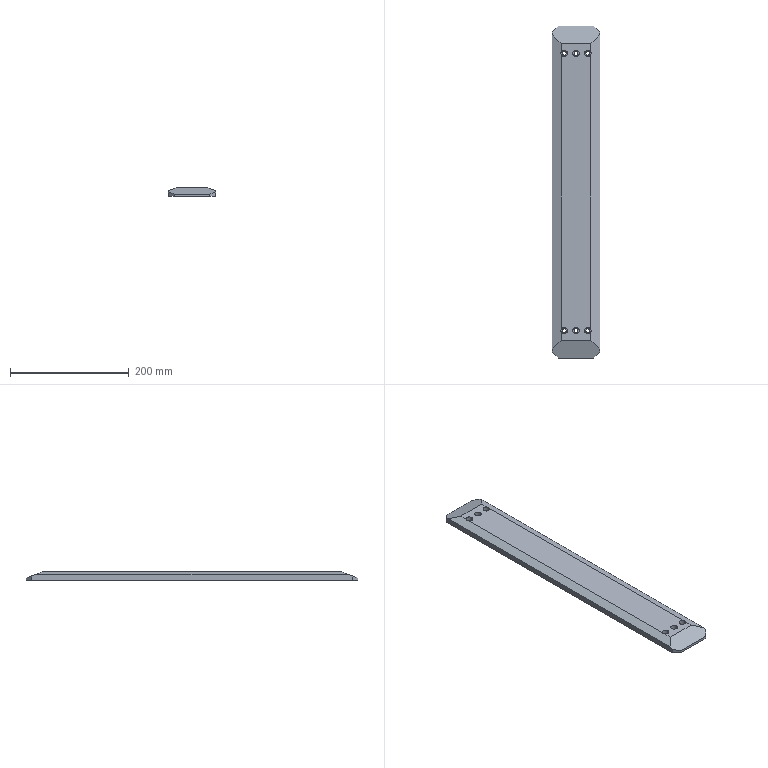Part | SolidWorks | features BaseBody 1 | 1 solid | 44 faces | box 80 x 560 x 15 mm | volume 596607 mm3 | cylinder 24 | plane 20 | commonest cylinder face diameters 6.6 x12 11 x12
STEP:
#1=CARTESIAN_POINT('',(14.5,-234.,6.));
#2=VERTEX_POINT('',#1);
#3=CARTESIAN_POINT('',(25.5,-234.,6.));
#4=VERTEX_POINT('',#3);
#5=CARTESIAN_POINT('',(20.,-234.,6.));
#6=DIRECTION('',(0.,0.,1.));
#7=DIRECTION('',(1.,0.,0.));
#8=AXIS2_PLACEMENT_3D('',#5,#6,#7);
#9=CIRCLE('',#8,5.5);
#10=EDGE_CURVE('',#2,#4,#9,.T.);
#11=ORIENTED_EDGE('',*,*,#10,.F.);
#12=CARTESIAN_POINT('',(14.5,-234.,15.));
#13=VERTEX_POINT('',#12);
#14=CARTESIAN_POINT('',(14.5,-234.,15.));
#15=DIRECTION('',(0.,0.,1.));
#16=VECTOR('',#15,1000.);
#17=LINE('',#14,#16);
#18=EDGE_CURVE('',#2,#13,#17,.T.);
#19=ORIENTED_EDGE('',*,*,#18,.T.);
#20=CARTESIAN_POINT('',(25.,-236.291,15.));
#21=VERTEX_POINT('',#20);
#22=CARTESIAN_POINT('',(20.,-234.,15.));
#23=DIRECTION('',(0.,0.,1.));
#24=DIRECTION('',(1.,0.,0.));
#25=AXIS2_PLACEMENT_3D('',#22,#23,#24);
#26=CIRCLE('',#25,5.5);
#27=EDGE_CURVE('',#13,#21,#26,.T.);
#28=ORIENTED_EDGE('',*,*,#27,.T.);
#29=CARTESIAN_POINT('',(25.5,-234.,14.818));
#30=VERTEX_POINT('',#29);
#31=CARTESIAN_POINT('',(25.,-236.291,15.));
#32=CARTESIAN_POINT('',(25.331,-235.57,14.88));
#33=CARTESIAN_POINT('',(25.5,-234.794,14.818));
#34=CARTESIAN_POINT('',(25.5,-234.,14.818));
#35=(BOUNDED_CURVE()B_SPLINE_CURVE(3,(#31,#32,#33,#34),.UNSPECIFIED.,.F.,.T.)B_SPLINE_CURVE_WITH_KNOTS((4,4),(2.712,3.142),.UNSPECIFIED.)CURVE()GEOMETRIC_REPRESENTATION_ITEM()RATIONAL_B_SPLINE_CURVE((1.,0.9847,0.9847,1.))REPRESENTATION_ITEM(''));
#36=EDGE_CURVE('',#21,#30,#35,.T.);
#37=ORIENTED_EDGE('',*,*,#36,.T.);
#38=CARTESIAN_POINT('',(25.5,-234.,15.));
#39=DIRECTION('',(0.,0.,1.));
#40=VECTOR('',#39,1000.);
#41=LINE('',#38,#40);
#42=EDGE_CURVE('',#4,#30,#41,.T.);
#43=ORIENTED_EDGE('',*,*,#42,.F.);
#44=EDGE_LOOP('',(#11,#19,#28,#37,#43));
#45=FACE_OUTER_BOUND('',#44,.T.);
#46=CARTESIAN_POINT('',(20.,-234.,15.));
#47=DIRECTION('',(0.,0.,1.));
#48=DIRECTION('',(1.,0.,0.));
#49=AXIS2_PLACEMENT_3D('',#46,#47,#48);
#50=CYLINDRICAL_SURFACE('',#49,5.5);
#51=ADVANCED_FACE('',(#45),#50,.F.);
#52=CARTESIAN_POINT('',(16.7,-234.,0.));
#53=VERTEX_POINT('',#52);
#54=CARTESIAN_POINT('',(23.3,-234.,0.));
#55=VERTEX_POINT('',#54);
#56=CARTESIAN_POINT('',(20.,-234.,0.));
#57=DIRECTION('',(0.,0.,1.));
#58=DIRECTION('',(1.,0.,0.));
#59=AXIS2_PLACEMENT_3D('',#56,#57,#58);
#60=CIRCLE('',#59,3.3);
#61=EDGE_CURVE('',#53,#55,#60,.T.);
#62=ORIENTED_EDGE('',*,*,#61,.F.);
#63=CARTESIAN_POINT('',(16.7,-234.,6.));
#64=VERTEX_POINT('',#63);
#65=CARTESIAN_POINT('',(16.7,-234.,15.));
#66=DIRECTION('',(0.,0.,1.));
#67=VECTOR('',#66,1000.);
#68=LINE('',#65,#67);
#69=EDGE_CURVE('',#53,#64,#68,.T.);
#70=ORIENTED_EDGE('',*,*,#69,.T.);
#71=CARTESIAN_POINT('',(23.3,-234.,6.));
#72=VERTEX_POINT('',#71);
#73=CARTESIAN_POINT('',(20.,-234.,6.));
#74=DIRECTION('',(0.,0.,1.));
#75=DIRECTION('',(1.,0.,0.));
#76=AXIS2_PLACEMENT_3D('',#73,#74,#75);
#77=CIRCLE('',#76,3.3);
#78=EDGE_CURVE('',#64,#72,#77,.T.);
#79=ORIENTED_EDGE('',*,*,#78,.T.);
#80=CARTESIAN_POINT('',(23.3,-234.,15.));
#81=DIRECTION('',(0.,0.,1.));
#82=VECTOR('',#81,1000.);
#83=LINE('',#80,#82);
#84=EDGE_CURVE('',#55,#72,#83,.T.);
#85=ORIENTED_EDGE('',*,*,#84,.F.);
#86=EDGE_LOOP('',(#62,#70,#79,#85));
#87=FACE_OUTER_BOUND('',#86,.T.);
#88=CARTESIAN_POINT('',(20.,-234.,15.));
#89=DIRECTION('',(0.,0.,1.));
#90=DIRECTION('',(1.,0.,0.));
#91=AXIS2_PLACEMENT_3D('',#88,#89,#90);
#92=CYLINDRICAL_SURFACE('',#91,3.3);
#93=ADVANCED_FACE('',(#87),#92,.F.);
#94=CARTESIAN_POINT('',(-5.5,-234.,6.));
#95=VERTEX_POINT('',#94);
#96=CARTESIAN_POINT('',(5.5,-234.,6.));
#97=VERTEX_POINT('',#96);
#98=CARTESIAN_POINT('',(0.,-234.,6.));
#99=DIRECTION('',(0.,0.,1.));
#100=DIRECTION('',(1.,0.,0.));
#101=AXIS2_PLACEMENT_3D('',#98,#99,#100);
#102=CIRCLE('',#101,5.5);
#103=EDGE_CURVE('',#95,#97,#102,.T.);
#104=ORIENTED_EDGE('',*,*,#103,.F.);
#105=CARTESIAN_POINT('',(-5.5,-234.,15.));
#106=VERTEX_POINT('',#105);
#107=CARTESIAN_POINT('',(-5.5,-234.,15.));
#108=DIRECTION('',(0.,0.,1.));
#109=VECTOR('',#108,1000.);
#110=LINE('',#107,#109);
#111=EDGE_CURVE('',#95,#106,#110,.T.);
#112=ORIENTED_EDGE('',*,*,#111,.T.);
#113=CARTESIAN_POINT('',(5.5,-234.,15.));
#114=VERTEX_POINT('',#113);
#115=CARTESIAN_POINT('',(0.,-234.,15.));
#116=DIRECTION('',(0.,0.,1.));
#117=DIRECTION('',(1.,0.,0.));
#118=AXIS2_PLACEMENT_3D('',#115,#116,#117);
#119=CIRCLE('',#118,5.5);
#120=EDGE_CURVE('',#106,#114,#119,.T.);
#121=ORIENTED_EDGE('',*,*,#120,.T.);
#122=CARTESIAN_POINT('',(5.5,-234.,15.));
#123=DIRECTION('',(0.,0.,1.));
#124=VECTOR('',#123,1000.);
#125=LINE('',#122,#124);
#126=EDGE_CURVE('',#97,#114,#125,.T.);
#127=ORIENTED_EDGE('',*,*,#126,.F.);
#128=EDGE_LOOP('',(#104,#112,#121,#127));
#129=FACE_OUTER_BOUND('',#128,.T.);
#130=CARTESIAN_POINT('',(0.,-234.,15.));
#131=DIRECTION('',(0.,0.,1.));
#132=DIRECTION('',(1.,0.,0.));
#133=AXIS2_PLACEMENT_3D('',#130,#131,#132);
#134=CYLINDRICAL_SURFACE('',#133,5.5);
#135=ADVANCED_FACE('',(#129),#134,.F.);
#136=CARTESIAN_POINT('',(-3.3,-234.,0.));
#137=VERTEX_POINT('',#136);
#138=CARTESIAN_POINT('',(3.3,-234.,0.));
#139=VERTEX_POINT('',#138);
#140=CARTESIAN_POINT('',(0.,-234.,0.));
#141=DIRECTION('',(0.,0.,1.));
#142=DIRECTION('',(1.,0.,0.));
#143=AXIS2_PLACEMENT_3D('',#140,#141,#142);
#144=CIRCLE('',#143,3.3);
#145=EDGE_CURVE('',#137,#139,#144,.T.);
#146=ORIENTED_EDGE('',*,*,#145,.F.);
#147=CARTESIAN_POINT('',(-3.3,-234.,6.));
#148=VERTEX_POINT('',#147);
#149=CARTESIAN_POINT('',(-3.3,-234.,15.));
#150=DIRECTION('',(0.,0.,1.));
#151=VECTOR('',#150,1000.);
#152=LINE('',#149,#151);
#153=EDGE_CURVE('',#137,#148,#152,.T.);
#154=ORIENTED_EDGE('',*,*,#153,.T.);
#155=CARTESIAN_POINT('',(3.3,-234.,6.));
#156=VERTEX_POINT('',#155);
#157=CARTESIAN_POINT('',(0.,-234.,6.));
#158=DIRECTION('',(0.,0.,1.));
#159=DIRECTION('',(1.,0.,0.));
#160=AXIS2_PLACEMENT_3D('',#157,#158,#159);
#161=CIRCLE('',#160,3.3);
#162=EDGE_CURVE('',#148,#156,#161,.T.);
#163=ORIENTED_EDGE('',*,*,#162,.T.);
#164=CARTESIAN_POINT('',(3.3,-234.,15.));
#165=DIRECTION('',(0.,0.,1.));
#166=VECTOR('',#165,1000.);
#167=LINE('',#164,#166);
#168=EDGE_CURVE('',#139,#156,#167,.T.);
#169=ORIENTED_EDGE('',*,*,#168,.F.);
#170=EDGE_LOOP('',(#146,#154,#163,#169));
#171=FACE_OUTER_BOUND('',#170,.T.);
#172=CARTESIAN_POINT('',(0.,-234.,15.));
#173=DIRECTION('',(0.,0.,1.));
#174=DIRECTION('',(1.,0.,0.));
#175=AXIS2_PLACEMENT_3D('',#172,#173,#174);
#176=CYLINDRICAL_SURFACE('',#175,3.3);
#177=ADVANCED_FACE('',(#171),#176,.F.);
#178=CARTESIAN_POINT('',(-25.5,-234.,6.));
#179=VERTEX_POINT('',#178);
#180=CARTESIAN_POINT('',(-14.5,-234.,6.));
#181=VERTEX_POINT('',#180);
#182=CARTESIAN_POINT('',(-20.,-234.,6.));
#183=DIRECTION('',(0.,0.,1.));
#184=DIRECTION('',(1.,0.,0.));
#185=AXIS2_PLACEMENT_3D('',#182,#183,#184);
#186=CIRCLE('',#185,5.5);
#187=EDGE_CURVE('',#179,#181,#186,.T.);
#188=ORIENTED_EDGE('',*,*,#187,.F.);
#189=CARTESIAN_POINT('',(-25.5,-234.,14.818));
#190=VERTEX_POINT('',#189);
#191=CARTESIAN_POINT('',(-25.5,-234.,15.));
#192=DIRECTION('',(0.,0.,1.));
#193=VECTOR('',#192,1000.);
#194=LINE('',#191,#193);
#195=EDGE_CURVE('',#179,#190,#194,.T.);
#196=ORIENTED_EDGE('',*,*,#195,.T.);
#197=CARTESIAN_POINT('',(-25.,-236.291,15.));
#198=VERTEX_POINT('',#197);
#199=CARTESIAN_POINT('',(-25.5,-234.,14.818));
#200=CARTESIAN_POINT('',(-25.5,-234.794,14.818));
#201=CARTESIAN_POINT('',(-25.331,-235.57,14.88));
#202=CARTESIAN_POINT('',(-25.,-236.291,15.));
#203=(BOUNDED_CURVE()B_SPLINE_CURVE(3,(#199,#200,#201,#202),.UNSPECIFIED.,.F.,.T.)B_SPLINE_CURVE_WITH_KNOTS((4,4),(3.142,3.571),.UNSPECIFIED.)CURVE()GEOMETRIC_REPRESENTATION_ITEM()RATIONAL_B_SPLINE_CURVE((1.,0.9847,0.9847,1.))REPRESENTATION_ITEM(''));
#204=EDGE_CURVE('',#190,#198,#203,.T.);
#205=ORIENTED_EDGE('',*,*,#204,.T.);
#206=CARTESIAN_POINT('',(-14.5,-234.,15.));
#207=VERTEX_POINT('',#206);
#208=CARTESIAN_POINT('',(-20.,-234.,15.));
#209=DIRECTION('',(0.,0.,1.));
#210=DIRECTION('',(1.,0.,0.));
#211=AXIS2_PLACEMENT_3D('',#208,#209,#210);
#212=CIRCLE('',#211,5.5);
#213=EDGE_CURVE('',#198,#207,#212,.T.);
#214=ORIENTED_EDGE('',*,*,#213,.T.);
#215=CARTESIAN_POINT('',(-14.5,-234.,15.));
#216=DIRECTION('',(0.,0.,1.));
#217=VECTOR('',#216,1000.);
#218=LINE('',#215,#217);
#219=EDGE_CURVE('',#181,#207,#218,.T.);
#220=ORIENTED_EDGE('',*,*,#219,.F.);
#221=EDGE_LOOP('',(#188,#196,#205,#214,#220));
#222=FACE_OUTER_BOUND('',#221,.T.);
#223=CARTESIAN_POINT('',(-20.,-234.,15.));
#224=DIRECTION('',(0.,0.,1.));
#225=DIRECTION('',(1.,0.,0.));
#226=AXIS2_PLACEMENT_3D('',#223,#224,#225);
#227=CYLINDRICAL_SURFACE('',#226,5.5);
#228=ADVANCED_FACE('',(#222),#227,.F.);
#229=CARTESIAN_POINT('',(-23.3,-234.,0.));
#230=VERTEX_POINT('',#229);
#231=CARTESIAN_POINT('',(-16.7,-234.,0.));
#232=VERTEX_POINT('',#231);
#233=CARTESIAN_POINT('',(-20.,-234.,0.));
#234=DIRECTION('',(0.,0.,1.));
#235=DIRECTION('',(1.,0.,0.));
#236=AXIS2_PLACEMENT_3D('',#233,#234,#235);
#237=CIRCLE('',#236,3.3);
#238=EDGE_CURVE('',#230,#232,#237,.T.);
#239=ORIENTED_EDGE('',*,*,#238,.F.);
#240=CARTESIAN_POINT('',(-23.3,-234.,6.));
#241=VERTEX_POINT('',#240);
#242=CARTESIAN_POINT('',(-23.3,-234.,15.));
#243=DIRECTION('',(0.,0.,1.));
#244=VECTOR('',#243,1000.);
#245=LINE('',#242,#244);
#246=EDGE_CURVE('',#230,#241,#245,.T.);
#247=ORIENTED_EDGE('',*,*,#246,.T.);
#248=CARTESIAN_POINT('',(-16.7,-234.,6.));
#249=VERTEX_POINT('',#248);
#250=CARTESIAN_POINT('',(-20.,-234.,6.));
#251=DIRECTION('',(0.,0.,1.));
#252=DIRECTION('',(1.,0.,0.));
#253=AXIS2_PLACEMENT_3D('',#250,#251,#252);
#254=CIRCLE('',#253,3.3);
#255=EDGE_CURVE('',#241,#249,#254,.T.);
#256=ORIENTED_EDGE('',*,*,#255,.T.);
#257=CARTESIAN_POINT('',(-16.7,-234.,15.));
#258=DIRECTION('',(0.,0.,1.));
#259=VECTOR('',#258,1000.);
#260=LINE('',#257,#259);
#261=EDGE_CURVE('',#232,#249,#260,.T.);
#262=ORIENTED_EDGE('',*,*,#261,.F.);
#263=EDGE_LOOP('',(#239,#247,#256,#262));
#264=FACE_OUTER_BOUND('',#263,.T.);
#265=CARTESIAN_POINT('',(-20.,-234.,15.));
#266=DIRECTION('',(0.,0.,1.));
#267=DIRECTION('',(1.,0.,0.));
#268=AXIS2_PLACEMENT_3D('',#265,#266,#267);
#269=CYLINDRICAL_SURFACE('',#268,3.3);
#270=ADVANCED_FACE('',(#264),#269,.F.);
#271=CARTESIAN_POINT('',(14.5,234.,6.));
#272=VERTEX_POINT('',#271);
#273=CARTESIAN_POINT('',(25.5,234.,6.));
#274=VERTEX_POINT('',#273);
#275=CARTESIAN_POINT('',(20.,234.,6.));
#276=DIRECTION('',(0.,0.,1.));
#277=DIRECTION('',(1.,0.,0.));
#278=AXIS2_PLACEMENT_3D('',#275,#276,#277);
#279=CIRCLE('',#278,5.5);
#280=EDGE_CURVE('',#272,#274,#279,.T.);
#281=ORIENTED_EDGE('',*,*,#280,.F.);
#282=CARTESIAN_POINT('',(14.5,234.,15.));
#283=VERTEX_POINT('',#282);
#284=CARTESIAN_POINT('',(14.5,234.,15.));
#285=DIRECTION('',(0.,0.,1.));
#286=VECTOR('',#285,1000.);
#287=LINE('',#284,#286);
#288=EDGE_CURVE('',#272,#283,#287,.T.);
#289=ORIENTED_EDGE('',*,*,#288,.T.);
#290=CARTESIAN_POINT('',(25.,231.709,15.));
#291=VERTEX_POINT('',#290);
#292=CARTESIAN_POINT('',(20.,234.,15.));
#293=DIRECTION('',(0.,0.,1.));
#294=DIRECTION('',(1.,0.,0.));
#295=AXIS2_PLACEMENT_3D('',#292,#293,#294);
#296=CIRCLE('',#295,5.5);
#297=EDGE_CURVE('',#283,#291,#296,.T.);
#298=ORIENTED_EDGE('',*,*,#297,.T.);
#299=CARTESIAN_POINT('',(25.5,234.,14.818));
#300=VERTEX_POINT('',#299);
#301=CARTESIAN_POINT('',(25.,231.709,15.));
#302=CARTESIAN_POINT('',(25.331,232.43,14.88));
#303=CARTESIAN_POINT('',(25.5,233.206,14.818));
#304=CARTESIAN_POINT('',(25.5,234.,14.818));
#305=(BOUNDED_CURVE()B_SPLINE_CURVE(3,(#301,#302,#303,#304),.UNSPECIFIED.,.F.,.T.)B_SPLINE_CURVE_WITH_KNOTS((4,4),(2.712,3.142),.UNSPECIFIED.)CURVE()GEOMETRIC_REPRESENTATION_ITEM()RATIONAL_B_SPLINE_CURVE((1.,0.9847,0.9847,1.))REPRESENTATION_ITEM(''));
#306=EDGE_CURVE('',#291,#300,#305,.T.);
#307=ORIENTED_EDGE('',*,*,#306,.T.);
#308=CARTESIAN_POINT('',(25.5,234.,15.));
#309=DIRECTION('',(0.,0.,1.));
#310=VECTOR('',#309,1000.);
#311=LINE('',#308,#310);
#312=EDGE_CURVE('',#274,#300,#311,.T.);
#313=ORIENTED_EDGE('',*,*,#312,.F.);
#314=EDGE_LOOP('',(#281,#289,#298,#307,#313));
#315=FACE_OUTER_BOUND('',#314,.T.);
#316=CARTESIAN_POINT('',(20.,234.,15.));
#317=DIRECTION('',(0.,0.,1.));
#318=DIRECTION('',(1.,0.,0.));
#319=AXIS2_PLACEMENT_3D('',#316,#317,#318);
#320=CYLINDRICAL_SURFACE('',#319,5.5);
#321=ADVANCED_FACE('',(#315),#320,.F.);
#322=CARTESIAN_POINT('',(16.7,234.,0.));
#323=VERTEX_POINT('',#322);
#324=CARTESIAN_POINT('',(23.3,234.,0.));
#325=VERTEX_POINT('',#324);
#326=CARTESIAN_POINT('',(20.,234.,0.));
#327=DIRECTION('',(0.,0.,1.));
#328=DIRECTION('',(1.,0.,0.));
#329=AXIS2_PLACEMENT_3D('',#326,#327,#328);
#330=CIRCLE('',#329,3.3);
#331=EDGE_CURVE('',#323,#325,#330,.T.);
#332=ORIENTED_EDGE('',*,*,#331,.F.);
#333=CARTESIAN_POINT('',(16.7,234.,6.));
#334=VERTEX_POINT('',#333);
#335=CARTESIAN_POINT('',(16.7,234.,15.));
#336=DIRECTION('',(0.,0.,1.));
#337=VECTOR('',#336,1000.);
#338=LINE('',#335,#337);
#339=EDGE_CURVE('',#323,#334,#338,.T.);
#340=ORIENTED_EDGE('',*,*,#339,.T.);
#341=CARTESIAN_POINT('',(23.3,234.,6.));
#342=VERTEX_POINT('',#341);
#343=CARTESIAN_POINT('',(20.,234.,6.));
#344=DIRECTION('',(0.,0.,1.));
#345=DIRECTION('',(1.,0.,0.));
#346=AXIS2_PLACEMENT_3D('',#343,#344,#345);
#347=CIRCLE('',#346,3.3);
#348=EDGE_CURVE('',#334,#342,#347,.T.);
#349=ORIENTED_EDGE('',*,*,#348,.T.);
#350=CARTESIAN_POINT('',(23.3,234.,15.));
#351=DIRECTION('',(0.,0.,1.));
#352=VECTOR('',#351,1000.);
#353=LINE('',#350,#352);
#354=EDGE_CURVE('',#325,#342,#353,.T.);
#355=ORIENTED_EDGE('',*,*,#354,.F.);
#356=EDGE_LOOP('',(#332,#340,#349,#355));
#357=FACE_OUTER_BOUND('',#356,.T.);
#358=CARTESIAN_POINT('',(20.,234.,15.));
#359=DIRECTION('',(0.,0.,1.));
#360=DIRECTION('',(1.,0.,0.));
#361=AXIS2_PLACEMENT_3D('',#358,#359,#360);
#362=CYLINDRICAL_SURFACE('',#361,3.3);
#363=ADVANCED_FACE('',(#357),#362,.F.);
#364=CARTESIAN_POINT('',(-5.5,234.,6.));
#365=VERTEX_POINT('',#364);
#366=CARTESIAN_POINT('',(5.5,234.,6.));
#367=VERTEX_POINT('',#366);
#368=CARTESIAN_POINT('',(0.,234.,6.));
#369=DIRECTION('',(0.,0.,1.));
#370=DIRECTION('',(1.,0.,0.));
#371=AXIS2_PLACEMENT_3D('',#368,#369,#370);
#372=CIRCLE('',#371,5.5);
#373=EDGE_CURVE('',#365,#367,#372,.T.);
#374=ORIENTED_EDGE('',*,*,#373,.F.);
#375=CARTESIAN_POINT('',(-5.5,234.,15.));
#376=VERTEX_POINT('',#375);
#377=CARTESIAN_POINT('',(-5.5,234.,15.));
#378=DIRECTION('',(0.,0.,1.));
#379=VECTOR('',#378,1000.);
#380=LINE('',#377,#379);
#381=EDGE_CURVE('',#365,#376,#380,.T.);
#382=ORIENTED_EDGE('',*,*,#381,.T.);
#383=CARTESIAN_POINT('',(5.5,234.,15.));
#384=VERTEX_POINT('',#383);
#385=CARTESIAN_POINT('',(0.,234.,15.));
#386=DIRECTION('',(0.,0.,1.));
#387=DIRECTION('',(1.,0.,0.));
#388=AXIS2_PLACEMENT_3D('',#385,#386,#387);
#389=CIRCLE('',#388,5.5);
#390=EDGE_CURVE('',#376,#384,#389,.T.);
#391=ORIENTED_EDGE('',*,*,#390,.T.);
#392=CARTESIAN_POINT('',(5.5,234.,15.));
#393=DIRECTION('',(0.,0.,1.));
#394=VECTOR('',#393,1000.);
#395=LINE('',#392,#394);
#396=EDGE_CURVE('',#367,#384,#395,.T.);
#397=ORIENTED_EDGE('',*,*,#396,.F.);
#398=EDGE_LOOP('',(#374,#382,#391,#397));
#399=FACE_OUTER_BOUND('',#398,.T.);
#400=CARTESIAN_POINT('',(0.,234.,15.));
#401=DIRECTION('',(0.,0.,1.));
#402=DIRECTION('',(1.,0.,0.));
#403=AXIS2_PLACEMENT_3D('',#400,#401,#402);
#404=CYLINDRICAL_SURFACE('',#403,5.5);
#405=ADVANCED_FACE('',(#399),#404,.F.);
#406=CARTESIAN_POINT('',(-3.3,234.,0.));
#407=VERTEX_POINT('',#406);
#408=CARTESIAN_POINT('',(3.3,234.,0.));
#409=VERTEX_POINT('',#408);
#410=CARTESIAN_POINT('',(0.,234.,0.));
#411=DIRECTION('',(0.,0.,1.));
#412=DIRECTION('',(1.,0.,0.));
#413=AXIS2_PLACEMENT_3D('',#410,#411,#412);
#414=CIRCLE('',#413,3.3);
#415=EDGE_CURVE('',#407,#409,#414,.T.);
#416=ORIENTED_EDGE('',*,*,#415,.F.);
#417=CARTESIAN_POINT('',(-3.3,234.,6.));
#418=VERTEX_POINT('',#417);
#419=CARTESIAN_POINT('',(-3.3,234.,15.));
#420=DIRECTION('',(0.,0.,1.));
#421=VECTOR('',#420,1000.);
#422=LINE('',#419,#421);
#423=EDGE_CURVE('',#407,#418,#422,.T.);
#424=ORIENTED_EDGE('',*,*,#423,.T.);
#425=CARTESIAN_POINT('',(3.3,234.,6.));
#426=VERTEX_POINT('',#425);
#427=CARTESIAN_POINT('',(0.,234.,6.));
#428=DIRECTION('',(0.,0.,1.));
#429=DIRECTION('',(1.,0.,0.));
#430=AXIS2_PLACEMENT_3D('',#427,#428,#429);
#431=CIRCLE('',#430,3.3);
#432=EDGE_CURVE('',#418,#426,#431,.T.);
#433=ORIENTED_EDGE('',*,*,#432,.T.);
#434=CARTESIAN_POINT('',(3.3,234.,15.));
#435=DIRECTION('',(0.,0.,1.));
#436=VECTOR('',#435,1000.);
#437=LINE('',#434,#436);
#438=EDGE_CURVE('',#409,#426,#437,.T.);
#439=ORIENTED_EDGE('',*,*,#438,.F.);
#440=EDGE_LOOP('',(#416,#424,#433,#439));
#441=FACE_OUTER_BOUND('',#440,.T.);
#442=CARTESIAN_POINT('',(0.,234.,15.));
#443=DIRECTION('',(0.,0.,1.));
#444=DIRECTION('',(1.,0.,0.));
#445=AXIS2_PLACEMENT_3D('',#442,#443,#444);
#446=CYLINDRICAL_SURFACE('',#445,3.3);
#447=ADVANCED_FACE('',(#441),#446,.F.);
#448=CARTESIAN_POINT('',(-25.5,234.,6.));
#449=VERTEX_POINT('',#448);
#450=CARTESIAN_POINT('',(-14.5,234.,6.));
#451=VERTEX_POINT('',#450);
#452=CARTESIAN_POINT('',(-20.,234.,6.));
#453=DIRECTION('',(0.,0.,1.));
#454=DIRECTION('',(1.,0.,0.));
#455=AXIS2_PLACEMENT_3D('',#452,#453,#454);
#456=CIRCLE('',#455,5.5);
#457=EDGE_CURVE('',#449,#451,#456,.T.);
#458=ORIENTED_EDGE('',*,*,#457,.F.);
#459=CARTESIAN_POINT('',(-25.5,234.,14.818));
#460=VERTEX_POINT('',#459);
#461=CARTESIAN_POINT('',(-25.5,234.,15.));
#462=DIRECTION('',(0.,0.,1.));
#463=VECTOR('',#462,1000.);
#464=LINE('',#461,#463);
#465=EDGE_CURVE('',#449,#460,#464,.T.);
#466=ORIENTED_EDGE('',*,*,#465,.T.);
#467=CARTESIAN_POINT('',(-25.,231.709,15.));
#468=VERTEX_POINT('',#467);
#469=CARTESIAN_POINT('',(-25.5,234.,14.818));
#470=CARTESIAN_POINT('',(-25.5,233.206,14.818));
#471=CARTESIAN_POINT('',(-25.331,232.43,14.88));
#472=CARTESIAN_POINT('',(-25.,231.709,15.));
#473=(BOUNDED_CURVE()B_SPLINE_CURVE(3,(#469,#470,#471,#472),.UNSPECIFIED.,.F.,.T.)B_SPLINE_CURVE_WITH_KNOTS((4,4),(3.142,3.571),.UNSPECIFIED.)CURVE()GEOMETRIC_REPRESENTATION_ITEM()RATIONAL_B_SPLINE_CURVE((1.,0.9847,0.9847,1.))REPRESENTATION_ITEM(''));
#474=EDGE_CURVE('',#460,#468,#473,.T.);
#475=ORIENTED_EDGE('',*,*,#474,.T.);
#476=CARTESIAN_POINT('',(-14.5,234.,15.));
#477=VERTEX_POINT('',#476);
#478=CARTESIAN_POINT('',(-20.,234.,15.));
#479=DIRECTION('',(0.,0.,1.));
#480=DIRECTION('',(1.,0.,0.));
#481=AXIS2_PLACEMENT_3D('',#478,#479,#480);
#482=CIRCLE('',#481,5.5);
#483=EDGE_CURVE('',#468,#477,#482,.T.);
#484=ORIENTED_EDGE('',*,*,#483,.T.);
#485=CARTESIAN_POINT('',(-14.5,234.,15.));
#486=DIRECTION('',(0.,0.,1.));
#487=VECTOR('',#486,1000.);
#488=LINE('',#485,#487);
#489=EDGE_CURVE('',#451,#477,#488,.T.);
#490=ORIENTED_EDGE('',*,*,#489,.F.);
#491=EDGE_LOOP('',(#458,#466,#475,#484,#490));
#492=FACE_OUTER_BOUND('',#491,.T.);
#493=CARTESIAN_POINT('',(-20.,234.,15.));
#494=DIRECTION('',(0.,0.,1.));
#495=DIRECTION('',(1.,0.,0.));
#496=AXIS2_PLACEMENT_3D('',#493,#494,#495);
#497=CYLINDRICAL_SURFACE('',#496,5.5);
#498=ADVANCED_FACE('',(#492),#497,.F.);
#499=CARTESIAN_POINT('',(-23.3,234.,0.));
#500=VERTEX_POINT('',#499);
#501=CARTESIAN_POINT('',(-16.7,234.,0.));
#502=VERTEX_POINT('',#501);
#503=CARTESIAN_POINT('',(-20.,234.,0.));
#504=DIRECTION('',(0.,0.,1.));
#505=DIRECTION('',(1.,0.,0.));
#506=AXIS2_PLACEMENT_3D('',#503,#504,#505);
#507=CIRCLE('',#506,3.3);
#508=EDGE_CURVE('',#500,#502,#507,.T.);
#509=ORIENTED_EDGE('',*,*,#508,.F.);
#510=CARTESIAN_POINT('',(-23.3,234.,6.));
#511=VERTEX_POINT('',#510);
#512=CARTESIAN_POINT('',(-23.3,234.,15.));
#513=DIRECTION('',(0.,0.,1.));
#514=VECTOR('',#513,1000.);
#515=LINE('',#512,#514);
#516=EDGE_CURVE('',#500,#511,#515,.T.);
#517=ORIENTED_EDGE('',*,*,#516,.T.);
#518=CARTESIAN_POINT('',(-16.7,234.,6.));
#519=VERTEX_POINT('',#518);
#520=CARTESIAN_POINT('',(-20.,234.,6.));
#521=DIRECTION('',(0.,0.,1.));
#522=DIRECTION('',(1.,0.,0.));
#523=AXIS2_PLACEMENT_3D('',#520,#521,#522);
#524=CIRCLE('',#523,3.3);
#525=EDGE_CURVE('',#511,#519,#524,.T.);
#526=ORIENTED_EDGE('',*,*,#525,.T.);
#527=CARTESIAN_POINT('',(-16.7,234.,15.));
#528=DIRECTION('',(0.,0.,1.));
#529=VECTOR('',#528,1000.);
#530=LINE('',#527,#529);
#531=EDGE_CURVE('',#502,#519,#530,.T.);
#532=ORIENTED_EDGE('',*,*,#531,.F.);
#533=EDGE_LOOP('',(#509,#517,#526,#532));
#534=FACE_OUTER_BOUND('',#533,.T.);
#535=CARTESIAN_POINT('',(-20.,234.,15.));
#536=DIRECTION('',(0.,0.,1.));
#537=DIRECTION('',(1.,0.,0.));
#538=AXIS2_PLACEMENT_3D('',#535,#536,#537);
#539=CYLINDRICAL_SURFACE('',#538,3.3);
#540=ADVANCED_FACE('',(#534),#539,.F.);
#541=CARTESIAN_POINT('',(40.,270.,7.721));
#542=VERTEX_POINT('',#541);
#543=CARTESIAN_POINT('',(40.,265.,9.54));
#544=VERTEX_POINT('',#543);
#545=CARTESIAN_POINT('',(40.,250.,15.));
#546=DIRECTION('',(0.,-0.9397,0.342));
#547=VECTOR('',#546,1000.);
#548=LINE('',#545,#547);
#549=EDGE_CURVE('',#542,#544,#548,.T.);
#550=ORIENTED_EDGE('',*,*,#549,.T.);
#551=CARTESIAN_POINT('',(40.,-265.,9.54));
#552=VERTEX_POINT('',#551);
#553=CARTESIAN_POINT('',(40.,-250.,9.54));
#554=DIRECTION('',(0.,-1.,0.));
#555=VECTOR('',#554,1000.);
#556=LINE('',#553,#555);
#557=EDGE_CURVE('',#544,#552,#556,.T.);
#558=ORIENTED_EDGE('',*,*,#557,.T.);
#559=CARTESIAN_POINT('',(40.,-270.,7.721));
#560=VERTEX_POINT('',#559);
#561=CARTESIAN_POINT('',(40.,-250.,15.));
#562=DIRECTION('',(0.,-0.9397,-0.342));
#563=VECTOR('',#562,1000.);
#564=LINE('',#561,#563);
#565=EDGE_CURVE('',#552,#560,#564,.T.);
#566=ORIENTED_EDGE('',*,*,#565,.T.);
#567=CARTESIAN_POINT('',(40.,-270.,0.));
#568=VERTEX_POINT('',#567);
#569=CARTESIAN_POINT('',(40.,-270.,15.));
#570=DIRECTION('',(0.,0.,-1.));
#571=VECTOR('',#570,1000.);
#572=LINE('',#569,#571);
#573=EDGE_CURVE('',#560,#568,#572,.T.);
#574=ORIENTED_EDGE('',*,*,#573,.T.);
#575=CARTESIAN_POINT('',(40.,270.,0.));
#576=VERTEX_POINT('',#575);
#577=CARTESIAN_POINT('',(40.,280.,0.));
#578=DIRECTION('',(0.,1.,0.));
#579=VECTOR('',#578,1000.);
#580=LINE('',#577,#579);
#581=EDGE_CURVE('',#568,#576,#580,.T.);
#582=ORIENTED_EDGE('',*,*,#581,.T.);
#583=CARTESIAN_POINT('',(40.,270.,15.));
#584=DIRECTION('',(0.,0.,1.));
#585=VECTOR('',#584,1000.);
#586=LINE('',#583,#585);
#587=EDGE_CURVE('',#576,#542,#586,.T.);
#588=ORIENTED_EDGE('',*,*,#587,.T.);
#589=EDGE_LOOP('',(#550,#558,#566,#574,#582,#588));
#590=FACE_OUTER_BOUND('',#589,.T.);
#591=CARTESIAN_POINT('',(40.,280.,15.));
#592=DIRECTION('',(-1.,0.,0.));
#593=DIRECTION('',(0.,-1.,0.));
#594=AXIS2_PLACEMENT_3D('',#591,#592,#593);
#595=PLANE('',#594);
#596=ADVANCED_FACE('',(#590),#595,.F.);
#597=CARTESIAN_POINT('',(-30.,280.,0.));
#598=VERTEX_POINT('',#597);
#599=CARTESIAN_POINT('',(-30.,280.,4.081));
#600=VERTEX_POINT('',#599);
#601=CARTESIAN_POINT('',(-30.,280.,15.));
#602=DIRECTION('',(0.,0.,1.));
#603=VECTOR('',#602,1000.);
#604=LINE('',#601,#603);
#605=EDGE_CURVE('',#598,#600,#604,.T.);
#606=ORIENTED_EDGE('',*,*,#605,.T.);
#607=CARTESIAN_POINT('',(30.,280.,4.081));
#608=VERTEX_POINT('',#607);
#609=CARTESIAN_POINT('',(30.,280.,4.081));
#610=DIRECTION('',(1.,0.,0.));
#611=VECTOR('',#610,1000.);
#612=LINE('',#609,#611);
#613=EDGE_CURVE('',#600,#608,#612,.T.);
#614=ORIENTED_EDGE('',*,*,#613,.T.);
#615=CARTESIAN_POINT('',(30.,280.,0.));
#616=VERTEX_POINT('',#615);
#617=CARTESIAN_POINT('',(30.,280.,15.));
#618=DIRECTION('',(0.,0.,-1.));
#619=VECTOR('',#618,1000.);
#620=LINE('',#617,#619);
#621=EDGE_CURVE('',#608,#616,#620,.T.);
#622=ORIENTED_EDGE('',*,*,#621,.T.);
#623=CARTESIAN_POINT('',(-40.,280.,0.));
#624=DIRECTION('',(-1.,0.,0.));
#625=VECTOR('',#624,1000.);
#626=LINE('',#623,#625);
#627=EDGE_CURVE('',#616,#598,#626,.T.);
#628=ORIENTED_EDGE('',*,*,#627,.T.);
#629=EDGE_LOOP('',(#606,#614,#622,#628));
#630=FACE_OUTER_BOUND('',#629,.T.);
#631=CARTESIAN_POINT('',(-40.,280.,15.));
#632=DIRECTION('',(0.,-1.,0.));
#633=DIRECTION('',(0.,0.,-1.));
#634=AXIS2_PLACEMENT_3D('',#631,#632,#633);
#635=PLANE('',#634);
#636=ADVANCED_FACE('',(#630),#635,.F.);
#637=CARTESIAN_POINT('',(-40.,-270.,7.721));
#638=VERTEX_POINT('',#637);
#639=CARTESIAN_POINT('',(-40.,-265.,9.54));
#640=VERTEX_POINT('',#639);
#641=CARTESIAN_POINT('',(-40.,-250.,15.));
#642=DIRECTION('',(0.,0.9397,0.342));
#643=VECTOR('',#642,1000.);
#644=LINE('',#641,#643);
#645=EDGE_CURVE('',#638,#640,#644,.T.);
#646=ORIENTED_EDGE('',*,*,#645,.T.);
#647=CARTESIAN_POINT('',(-40.,265.,9.54));
#648=VERTEX_POINT('',#647);
#649=CARTESIAN_POINT('',(-40.,250.,9.54));
#650=DIRECTION('',(0.,1.,0.));
#651=VECTOR('',#650,1000.);
#652=LINE('',#649,#651);
#653=EDGE_CURVE('',#640,#648,#652,.T.);
#654=ORIENTED_EDGE('',*,*,#653,.T.);
#655=CARTESIAN_POINT('',(-40.,270.,7.721));
#656=VERTEX_POINT('',#655);
#657=CARTESIAN_POINT('',(-40.,250.,15.));
#658=DIRECTION('',(0.,0.9397,-0.342));
#659=VECTOR('',#658,1000.);
#660=LINE('',#657,#659);
#661=EDGE_CURVE('',#648,#656,#660,.T.);
#662=ORIENTED_EDGE('',*,*,#661,.T.);
#663=CARTESIAN_POINT('',(-40.,270.,0.));
#664=VERTEX_POINT('',#663);
#665=CARTESIAN_POINT('',(-40.,270.,15.));
#666=DIRECTION('',(0.,0.,-1.));
#667=VECTOR('',#666,1000.);
#668=LINE('',#665,#667);
#669=EDGE_CURVE('',#656,#664,#668,.T.);
#670=ORIENTED_EDGE('',*,*,#669,.T.);
#671=CARTESIAN_POINT('',(-40.,-270.,0.));
#672=VERTEX_POINT('',#671);
#673=CARTESIAN_POINT('',(-40.,280.,0.));
#674=DIRECTION('',(0.,-1.,0.));
#675=VECTOR('',#674,1000.);
#676=LINE('',#673,#675);
#677=EDGE_CURVE('',#664,#672,#676,.T.);
#678=ORIENTED_EDGE('',*,*,#677,.T.);
#679=CARTESIAN_POINT('',(-40.,-270.,15.));
#680=DIRECTION('',(0.,0.,1.));
#681=VECTOR('',#680,1000.);
#682=LINE('',#679,#681);
#683=EDGE_CURVE('',#672,#638,#682,.T.);
#684=ORIENTED_EDGE('',*,*,#683,.T.);
#685=EDGE_LOOP('',(#646,#654,#662,#670,#678,#684));
#686=FACE_OUTER_BOUND('',#685,.T.);
#687=CARTESIAN_POINT('',(-40.,280.,15.));
#688=DIRECTION('',(1.,0.,0.));
#689=DIRECTION('',(0.,1.,0.));
#690=AXIS2_PLACEMENT_3D('',#687,#688,#689);
#691=PLANE('',#690);
#692=ADVANCED_FACE('',(#686),#691,.F.);
#693=CARTESIAN_POINT('',(30.,-280.,0.));
#694=VERTEX_POINT('',#693);
#695=CARTESIAN_POINT('',(30.,-280.,4.081));
#696=VERTEX_POINT('',#695);
#697=CARTESIAN_POINT('',(30.,-280.,15.));
#698=DIRECTION('',(0.,0.,1.));
#699=VECTOR('',#698,1000.);
#700=LINE('',#697,#699);
#701=EDGE_CURVE('',#694,#696,#700,.T.);
#702=ORIENTED_EDGE('',*,*,#701,.T.);
#703=CARTESIAN_POINT('',(-30.,-280.,4.081));
#704=VERTEX_POINT('',#703);
#705=CARTESIAN_POINT('',(-30.,-280.,4.081));
#706=DIRECTION('',(-1.,0.,0.));
#707=VECTOR('',#706,1000.);
#708=LINE('',#705,#707);
#709=EDGE_CURVE('',#696,#704,#708,.T.);
#710=ORIENTED_EDGE('',*,*,#709,.T.);
#711=CARTESIAN_POINT('',(-30.,-280.,0.));
#712=VERTEX_POINT('',#711);
#713=CARTESIAN_POINT('',(-30.,-280.,15.));
#714=DIRECTION('',(0.,0.,-1.));
#715=VECTOR('',#714,1000.);
#716=LINE('',#713,#715);
#717=EDGE_CURVE('',#704,#712,#716,.T.);
#718=ORIENTED_EDGE('',*,*,#717,.T.);
#719=CARTESIAN_POINT('',(-40.,-280.,0.));
#720=DIRECTION('',(1.,0.,0.));
#721=VECTOR('',#720,1000.);
#722=LINE('',#719,#721);
#723=EDGE_CURVE('',#712,#694,#722,.T.);
#724=ORIENTED_EDGE('',*,*,#723,.T.);
#725=EDGE_LOOP('',(#702,#710,#718,#724));
#726=FACE_OUTER_BOUND('',#725,.T.);
#727=CARTESIAN_POINT('',(-40.,-280.,15.));
#728=DIRECTION('',(0.,1.,0.));
#729=DIRECTION('',(0.,0.,1.));
#730=AXIS2_PLACEMENT_3D('',#727,#728,#729);
#731=PLANE('',#730);
#732=ADVANCED_FACE('',(#726),#731,.F.);
#733=CARTESIAN_POINT('',(25.,-231.709,15.));
#734=VERTEX_POINT('',#733);
#735=CARTESIAN_POINT('',(20.,-234.,15.));
#736=DIRECTION('',(0.,0.,1.));
#737=DIRECTION('',(1.,0.,0.));
#738=AXIS2_PLACEMENT_3D('',#735,#736,#737);
#739=CIRCLE('',#738,5.5);
#740=EDGE_CURVE('',#734,#13,#739,.T.);
#741=ORIENTED_EDGE('',*,*,#740,.F.);
#742=CARTESIAN_POINT('',(25.,250.,15.));
#743=DIRECTION('',(0.,1.,0.));
#744=VECTOR('',#743,1000.);
#745=LINE('',#742,#744);
#746=EDGE_CURVE('',#734,#291,#745,.T.);
#747=ORIENTED_EDGE('',*,*,#746,.T.);
#748=ORIENTED_EDGE('',*,*,#297,.F.);
#749=CARTESIAN_POINT('',(25.,236.291,15.));
#750=VERTEX_POINT('',#749);
#751=CARTESIAN_POINT('',(20.,234.,15.));
#752=DIRECTION('',(0.,0.,1.));
#753=DIRECTION('',(1.,0.,0.));
#754=AXIS2_PLACEMENT_3D('',#751,#752,#753);
#755=CIRCLE('',#754,5.5);
#756=EDGE_CURVE('',#750,#283,#755,.T.);
#757=ORIENTED_EDGE('',*,*,#756,.F.);
#758=CARTESIAN_POINT('',(25.,250.,15.));
#759=VERTEX_POINT('',#758);
#760=CARTESIAN_POINT('',(25.,250.,15.));
#761=DIRECTION('',(0.,1.,0.));
#762=VECTOR('',#761,1000.);
#763=LINE('',#760,#762);
#764=EDGE_CURVE('',#750,#759,#763,.T.);
#765=ORIENTED_EDGE('',*,*,#764,.T.);
#766=CARTESIAN_POINT('',(-25.,250.,15.));
#767=VERTEX_POINT('',#766);
#768=CARTESIAN_POINT('',(-30.,250.,15.));
#769=DIRECTION('',(-1.,0.,0.));
#770=VECTOR('',#769,1000.);
#771=LINE('',#768,#770);
#772=EDGE_CURVE('',#759,#767,#771,.T.);
#773=ORIENTED_EDGE('',*,*,#772,.T.);
#774=CARTESIAN_POINT('',(-25.,236.291,15.));
#775=VERTEX_POINT('',#774);
#776=CARTESIAN_POINT('',(-25.,-250.,15.));
#777=DIRECTION('',(0.,-1.,0.));
#778=VECTOR('',#777,1000.);
#779=LINE('',#776,#778);
#780=EDGE_CURVE('',#767,#775,#779,.T.);
#781=ORIENTED_EDGE('',*,*,#780,.T.);
#782=CARTESIAN_POINT('',(-20.,234.,15.));
#783=DIRECTION('',(0.,0.,1.));
#784=DIRECTION('',(1.,0.,0.));
#785=AXIS2_PLACEMENT_3D('',#782,#783,#784);
#786=CIRCLE('',#785,5.5);
#787=EDGE_CURVE('',#477,#775,#786,.T.);
#788=ORIENTED_EDGE('',*,*,#787,.F.);
#789=ORIENTED_EDGE('',*,*,#483,.F.);
#790=CARTESIAN_POINT('',(-25.,-231.709,15.));
#791=VERTEX_POINT('',#790);
#792=CARTESIAN_POINT('',(-25.,-250.,15.));
#793=DIRECTION('',(0.,-1.,0.));
#794=VECTOR('',#793,1000.);
#795=LINE('',#792,#794);
#796=EDGE_CURVE('',#468,#791,#795,.T.);
#797=ORIENTED_EDGE('',*,*,#796,.T.);
#798=CARTESIAN_POINT('',(-20.,-234.,15.));
#799=DIRECTION('',(0.,0.,1.));
#800=DIRECTION('',(1.,0.,0.));
#801=AXIS2_PLACEMENT_3D('',#798,#799,#800);
#802=CIRCLE('',#801,5.5);
#803=EDGE_CURVE('',#207,#791,#802,.T.);
#804=ORIENTED_EDGE('',*,*,#803,.F.);
#805=ORIENTED_EDGE('',*,*,#213,.F.);
#806=CARTESIAN_POINT('',(-25.,-250.,15.));
#807=VERTEX_POINT('',#806);
#808=CARTESIAN_POINT('',(-25.,-250.,15.));
#809=DIRECTION('',(0.,-1.,0.));
#810=VECTOR('',#809,1000.);
#811=LINE('',#808,#810);
#812=EDGE_CURVE('',#198,#807,#811,.T.);
#813=ORIENTED_EDGE('',*,*,#812,.T.);
#814=CARTESIAN_POINT('',(25.,-250.,15.));
#815=VERTEX_POINT('',#814);
#816=CARTESIAN_POINT('',(30.,-250.,15.));
#817=DIRECTION('',(1.,0.,0.));
#818=VECTOR('',#817,1000.);
#819=LINE('',#816,#818);
#820=EDGE_CURVE('',#807,#815,#819,.T.);
#821=ORIENTED_EDGE('',*,*,#820,.T.);
#822=CARTESIAN_POINT('',(25.,250.,15.));
#823=DIRECTION('',(0.,1.,0.));
#824=VECTOR('',#823,1000.);
#825=LINE('',#822,#824);
#826=EDGE_CURVE('',#815,#21,#825,.T.);
#827=ORIENTED_EDGE('',*,*,#826,.T.);
#828=ORIENTED_EDGE('',*,*,#27,.F.);
#829=EDGE_LOOP('',(#741,#747,#748,#757,#765,#773,#781,#788,#789,#797,#804,#805,#813,#821,#827,#828));
#830=FACE_OUTER_BOUND('',#829,.T.);
#831=CARTESIAN_POINT('',(0.,-234.,15.));
#832=DIRECTION('',(0.,0.,1.));
#833=DIRECTION('',(1.,0.,0.));
#834=AXIS2_PLACEMENT_3D('',#831,#832,#833);
#835=CIRCLE('',#834,5.5);
#836=EDGE_CURVE('',#114,#106,#835,.T.);
#837=ORIENTED_EDGE('',*,*,#836,.F.);
#838=ORIENTED_EDGE('',*,*,#120,.F.);
#839=EDGE_LOOP('',(#837,#838));
#840=FACE_BOUND('',#839,.T.);
#841=CARTESIAN_POINT('',(0.,234.,15.));
#842=DIRECTION('',(0.,0.,1.));
#843=DIRECTION('',(1.,0.,0.));
#844=AXIS2_PLACEMENT_3D('',#841,#842,#843);
#845=CIRCLE('',#844,5.5);
#846=EDGE_CURVE('',#384,#376,#845,.T.);
#847=ORIENTED_EDGE('',*,*,#846,.F.);
#848=ORIENTED_EDGE('',*,*,#390,.F.);
#849=EDGE_LOOP('',(#847,#848));
#850=FACE_BOUND('',#849,.T.);
#851=CARTESIAN_POINT('',(0.,0.,15.));
#852=DIRECTION('',(0.,0.,1.));
#853=DIRECTION('',(1.,0.,0.));
#854=AXIS2_PLACEMENT_3D('',#851,#852,#853);
#855=PLANE('',#854);
#856=ADVANCED_FACE('',(#830,#840,#850),#855,.T.);
#857=CARTESIAN_POINT('',(20.,-234.,0.));
#858=DIRECTION('',(0.,0.,1.));
#859=DIRECTION('',(1.,0.,0.));
#860=AXIS2_PLACEMENT_3D('',#857,#858,#859);
#861=CIRCLE('',#860,3.3);
#862=EDGE_CURVE('',#55,#53,#861,.T.);
#863=ORIENTED_EDGE('',*,*,#862,.T.);
#864=ORIENTED_EDGE('',*,*,#61,.T.);
#865=EDGE_LOOP('',(#863,#864));
#866=FACE_BOUND('',#865,.T.);
#867=CARTESIAN_POINT('',(0.,-234.,0.));
#868=DIRECTION('',(0.,0.,1.));
#869=DIRECTION('',(1.,0.,0.));
#870=AXIS2_PLACEMENT_3D('',#867,#868,#869);
#871=CIRCLE('',#870,3.3);
#872=EDGE_CURVE('',#139,#137,#871,.T.);
#873=ORIENTED_EDGE('',*,*,#872,.T.);
#874=ORIENTED_EDGE('',*,*,#145,.T.);
#875=EDGE_LOOP('',(#873,#874));
#876=FACE_BOUND('',#875,.T.);
#877=CARTESIAN_POINT('',(-20.,-234.,0.));
#878=DIRECTION('',(0.,0.,1.));
#879=DIRECTION('',(1.,0.,0.));
#880=AXIS2_PLACEMENT_3D('',#877,#878,#879);
#881=CIRCLE('',#880,3.3);
#882=EDGE_CURVE('',#232,#230,#881,.T.);
#883=ORIENTED_EDGE('',*,*,#882,.T.);
#884=ORIENTED_EDGE('',*,*,#238,.T.);
#885=EDGE_LOOP('',(#883,#884));
#886=FACE_BOUND('',#885,.T.);
#887=CARTESIAN_POINT('',(20.,234.,0.));
#888=DIRECTION('',(0.,0.,1.));
#889=DIRECTION('',(1.,0.,0.));
#890=AXIS2_PLACEMENT_3D('',#887,#888,#889);
#891=CIRCLE('',#890,3.3);
#892=EDGE_CURVE('',#325,#323,#891,.T.);
#893=ORIENTED_EDGE('',*,*,#892,.T.);
#894=ORIENTED_EDGE('',*,*,#331,.T.);
#895=EDGE_LOOP('',(#893,#894));
#896=FACE_BOUND('',#895,.T.);
#897=CARTESIAN_POINT('',(0.,234.,0.));
#898=DIRECTION('',(0.,0.,1.));
#899=DIRECTION('',(1.,0.,0.));
#900=AXIS2_PLACEMENT_3D('',#897,#898,#899);
#901=CIRCLE('',#900,3.3);
#902=EDGE_CURVE('',#409,#407,#901,.T.);
#903=ORIENTED_EDGE('',*,*,#902,.T.);
#904=ORIENTED_EDGE('',*,*,#415,.T.);
#905=EDGE_LOOP('',(#903,#904));
#906=FACE_BOUND('',#905,.T.);
#907=CARTESIAN_POINT('',(-20.,234.,0.));
#908=DIRECTION('',(0.,0.,1.));
#909=DIRECTION('',(1.,0.,0.));
#910=AXIS2_PLACEMENT_3D('',#907,#908,#909);
#911=CIRCLE('',#910,3.3);
#912=EDGE_CURVE('',#502,#500,#911,.T.);
#913=ORIENTED_EDGE('',*,*,#912,.T.);
#914=ORIENTED_EDGE('',*,*,#508,.T.);
#915=EDGE_LOOP('',(#913,#914));
#916=FACE_BOUND('',#915,.T.);
#917=ORIENTED_EDGE('',*,*,#581,.F.);
#918=CARTESIAN_POINT('',(40.,-270.,0.));
#919=DIRECTION('',(-0.7071,-0.7071,0.));
#920=VECTOR('',#919,1000.);
#921=LINE('',#918,#920);
#922=EDGE_CURVE('',#568,#694,#921,.T.);
#923=ORIENTED_EDGE('',*,*,#922,.T.);
#924=ORIENTED_EDGE('',*,*,#723,.F.);
#925=CARTESIAN_POINT('',(-30.,-280.,0.));
#926=DIRECTION('',(-0.7071,0.7071,0.));
#927=VECTOR('',#926,1000.);
#928=LINE('',#925,#927);
#929=EDGE_CURVE('',#712,#672,#928,.T.);
#930=ORIENTED_EDGE('',*,*,#929,.T.);
#931=ORIENTED_EDGE('',*,*,#677,.F.);
#932=CARTESIAN_POINT('',(-40.,270.,0.));
#933=DIRECTION('',(0.7071,0.7071,0.));
#934=VECTOR('',#933,1000.);
#935=LINE('',#932,#934);
#936=EDGE_CURVE('',#664,#598,#935,.T.);
#937=ORIENTED_EDGE('',*,*,#936,.T.);
#938=ORIENTED_EDGE('',*,*,#627,.F.);
#939=CARTESIAN_POINT('',(30.,280.,0.));
#940=DIRECTION('',(0.7071,-0.7071,0.));
#941=VECTOR('',#940,1000.);
#942=LINE('',#939,#941);
#943=EDGE_CURVE('',#616,#576,#942,.T.);
#944=ORIENTED_EDGE('',*,*,#943,.T.);
#945=EDGE_LOOP('',(#917,#923,#924,#930,#931,#937,#938,#944));
#946=FACE_OUTER_BOUND('',#945,.T.);
#947=CARTESIAN_POINT('',(0.,0.,0.));
#948=DIRECTION('',(0.,0.,1.));
#949=DIRECTION('',(1.,0.,0.));
#950=AXIS2_PLACEMENT_3D('',#947,#948,#949);
#951=PLANE('',#950);
#952=ADVANCED_FACE('',(#866,#876,#886,#896,#906,#916,#946),#951,.F.);
#953=ORIENTED_EDGE('',*,*,#573,.F.);
#954=CARTESIAN_POINT('',(41.242,-268.758,8.173));
#955=DIRECTION('',(-0.6848,-0.6848,-0.2492));
#956=VECTOR('',#955,1000.);
#957=LINE('',#954,#956);
#958=EDGE_CURVE('',#560,#696,#957,.T.);
#959=ORIENTED_EDGE('',*,*,#958,.T.);
#960=ORIENTED_EDGE('',*,*,#701,.F.);
#961=ORIENTED_EDGE('',*,*,#922,.F.);
#962=EDGE_LOOP('',(#953,#959,#960,#961));
#963=FACE_OUTER_BOUND('',#962,.T.);
#964=CARTESIAN_POINT('',(40.,-270.,15.));
#965=DIRECTION('',(-0.7071,0.7071,0.));
#966=DIRECTION('',(0.,0.,-1.));
#967=AXIS2_PLACEMENT_3D('',#964,#965,#966);
#968=PLANE('',#967);
#969=ADVANCED_FACE('',(#963),#968,.F.);
#970=ORIENTED_EDGE('',*,*,#717,.F.);
#971=CARTESIAN_POINT('',(-31.864,-278.136,4.759));
#972=DIRECTION('',(-0.6848,0.6848,0.2492));
#973=VECTOR('',#972,1000.);
#974=LINE('',#971,#973);
#975=EDGE_CURVE('',#704,#638,#974,.T.);
#976=ORIENTED_EDGE('',*,*,#975,.T.);
#977=ORIENTED_EDGE('',*,*,#683,.F.);
#978=ORIENTED_EDGE('',*,*,#929,.F.);
#979=EDGE_LOOP('',(#970,#976,#977,#978));
#980=FACE_OUTER_BOUND('',#979,.T.);
#981=CARTESIAN_POINT('',(-30.,-280.,15.));
#982=DIRECTION('',(0.7071,0.7071,0.));
#983=DIRECTION('',(0.,0.,-1.));
#984=AXIS2_PLACEMENT_3D('',#981,#982,#983);
#985=PLANE('',#984);
#986=ADVANCED_FACE('',(#980),#985,.F.);
#987=ORIENTED_EDGE('',*,*,#621,.F.);
#988=CARTESIAN_POINT('',(31.864,278.136,4.759));
#989=DIRECTION('',(0.6848,-0.6848,0.2492));
#990=VECTOR('',#989,1000.);
#991=LINE('',#988,#990);
#992=EDGE_CURVE('',#608,#542,#991,.T.);
#993=ORIENTED_EDGE('',*,*,#992,.T.);
#994=ORIENTED_EDGE('',*,*,#587,.F.);
#995=ORIENTED_EDGE('',*,*,#943,.F.);
#996=EDGE_LOOP('',(#987,#993,#994,#995));
#997=FACE_OUTER_BOUND('',#996,.T.);
#998=CARTESIAN_POINT('',(30.,280.,15.));
#999=DIRECTION('',(-0.7071,-0.7071,0.));
#1000=DIRECTION('',(0.,0.,-1.));
#1001=AXIS2_PLACEMENT_3D('',#998,#999,#1000);
#1002=PLANE('',#1001);
#1003=ADVANCED_FACE('',(#997),#1002,.F.);
#1004=ORIENTED_EDGE('',*,*,#669,.F.);
#1005=CARTESIAN_POINT('',(-41.242,268.758,8.173));
#1006=DIRECTION('',(0.6848,0.6848,-0.2492));
#1007=VECTOR('',#1006,1000.);
#1008=LINE('',#1005,#1007);
#1009=EDGE_CURVE('',#656,#600,#1008,.T.);
#1010=ORIENTED_EDGE('',*,*,#1009,.T.);
#1011=ORIENTED_EDGE('',*,*,#605,.F.);
#1012=ORIENTED_EDGE('',*,*,#936,.F.);
#1013=EDGE_LOOP('',(#1004,#1010,#1011,#1012));
#1014=FACE_OUTER_BOUND('',#1013,.T.);
#1015=CARTESIAN_POINT('',(-40.,270.,15.));
#1016=DIRECTION('',(0.7071,-0.7071,0.));
#1017=DIRECTION('',(0.,0.,-1.));
#1018=AXIS2_PLACEMENT_3D('',#1015,#1016,#1017);
#1019=PLANE('',#1018);
#1020=ADVANCED_FACE('',(#1014),#1019,.F.);
#1021=ORIENTED_EDGE('',*,*,#661,.F.);
#1022=CARTESIAN_POINT('',(-13.277,238.277,19.267));
#1023=DIRECTION('',(0.6848,-0.6848,0.2492));
#1024=VECTOR('',#1023,1000.);
#1025=LINE('',#1022,#1024);
#1026=EDGE_CURVE('',#648,#767,#1025,.T.);
#1027=ORIENTED_EDGE('',*,*,#1026,.T.);
#1028=ORIENTED_EDGE('',*,*,#772,.F.);
#1029=CARTESIAN_POINT('',(13.277,238.277,19.267));
#1030=DIRECTION('',(0.6848,0.6848,-0.2492));
#1031=VECTOR('',#1030,1000.);
#1032=LINE('',#1029,#1031);
#1033=EDGE_CURVE('',#759,#544,#1032,.T.);
#1034=ORIENTED_EDGE('',*,*,#1033,.T.);
#1035=ORIENTED_EDGE('',*,*,#549,.F.);
#1036=ORIENTED_EDGE('',*,*,#992,.F.);
#1037=ORIENTED_EDGE('',*,*,#613,.F.);
#1038=ORIENTED_EDGE('',*,*,#1009,.F.);
#1039=EDGE_LOOP('',(#1021,#1027,#1028,#1034,#1035,#1036,#1037,#1038));
#1040=FACE_OUTER_BOUND('',#1039,.T.);
#1041=CARTESIAN_POINT('',(0.,250.,15.));
#1042=DIRECTION('',(0.,0.342,0.9397));
#1043=DIRECTION('',(1.,0.,0.));
#1044=AXIS2_PLACEMENT_3D('',#1041,#1042,#1043);
#1045=PLANE('',#1044);
#1046=ADVANCED_FACE('',(#1040),#1045,.T.);
#1047=ORIENTED_EDGE('',*,*,#820,.F.);
#1048=CARTESIAN_POINT('',(-13.277,-238.277,19.267));
#1049=DIRECTION('',(-0.6848,-0.6848,-0.2492));
#1050=VECTOR('',#1049,1000.);
#1051=LINE('',#1048,#1050);
#1052=EDGE_CURVE('',#807,#640,#1051,.T.);
#1053=ORIENTED_EDGE('',*,*,#1052,.T.);
#1054=ORIENTED_EDGE('',*,*,#645,.F.);
#1055=ORIENTED_EDGE('',*,*,#975,.F.);
#1056=ORIENTED_EDGE('',*,*,#709,.F.);
#1057=ORIENTED_EDGE('',*,*,#958,.F.);
#1058=ORIENTED_EDGE('',*,*,#565,.F.);
#1059=CARTESIAN_POINT('',(13.277,-238.277,19.267));
#1060=DIRECTION('',(-0.6848,0.6848,0.2492));
#1061=VECTOR('',#1060,1000.);
#1062=LINE('',#1059,#1061);
#1063=EDGE_CURVE('',#552,#815,#1062,.T.);
#1064=ORIENTED_EDGE('',*,*,#1063,.T.);
#1065=EDGE_LOOP('',(#1047,#1053,#1054,#1055,#1056,#1057,#1058,#1064));
#1066=FACE_OUTER_BOUND('',#1065,.T.);
#1067=CARTESIAN_POINT('',(0.,-250.,15.));
#1068=DIRECTION('',(0.,-0.342,0.9397));
#1069=DIRECTION('',(-1.,0.,0.));
#1070=AXIS2_PLACEMENT_3D('',#1067,#1068,#1069);
#1071=PLANE('',#1070);
#1072=ADVANCED_FACE('',(#1066),#1071,.T.);
#1073=CARTESIAN_POINT('',(-25.,-231.709,15.));
#1074=CARTESIAN_POINT('',(-25.331,-232.43,14.88));
#1075=CARTESIAN_POINT('',(-25.5,-233.206,14.818));
#1076=CARTESIAN_POINT('',(-25.5,-234.,14.818));
#1077=(BOUNDED_CURVE()B_SPLINE_CURVE(3,(#1073,#1074,#1075,#1076),.UNSPECIFIED.,.F.,.T.)B_SPLINE_CURVE_WITH_KNOTS((4,4),(2.712,3.142),.UNSPECIFIED.)CURVE()GEOMETRIC_REPRESENTATION_ITEM()RATIONAL_B_SPLINE_CURVE((1.,0.9847,0.9847,1.))REPRESENTATION_ITEM(''));
#1078=EDGE_CURVE('',#791,#190,#1077,.T.);
#1079=ORIENTED_EDGE('',*,*,#1078,.F.);
#1080=ORIENTED_EDGE('',*,*,#796,.F.);
#1081=ORIENTED_EDGE('',*,*,#474,.F.);
#1082=CARTESIAN_POINT('',(-25.,236.291,15.));
#1083=CARTESIAN_POINT('',(-25.331,235.57,14.88));
#1084=CARTESIAN_POINT('',(-25.5,234.794,14.818));
#1085=CARTESIAN_POINT('',(-25.5,234.,14.818));
#1086=(BOUNDED_CURVE()B_SPLINE_CURVE(3,(#1082,#1083,#1084,#1085),.UNSPECIFIED.,.F.,.T.)B_SPLINE_CURVE_WITH_KNOTS((4,4),(2.712,3.142),.UNSPECIFIED.)CURVE()GEOMETRIC_REPRESENTATION_ITEM()RATIONAL_B_SPLINE_CURVE((1.,0.9847,0.9847,1.))REPRESENTATION_ITEM(''));
#1087=EDGE_CURVE('',#775,#460,#1086,.T.);
#1088=ORIENTED_EDGE('',*,*,#1087,.F.);
#1089=ORIENTED_EDGE('',*,*,#780,.F.);
#1090=ORIENTED_EDGE('',*,*,#1026,.F.);
#1091=ORIENTED_EDGE('',*,*,#653,.F.);
#1092=ORIENTED_EDGE('',*,*,#1052,.F.);
#1093=ORIENTED_EDGE('',*,*,#812,.F.);
#1094=ORIENTED_EDGE('',*,*,#204,.F.);
#1095=EDGE_LOOP('',(#1079,#1080,#1081,#1088,#1089,#1090,#1091,#1092,#1093,#1094));
#1096=FACE_OUTER_BOUND('',#1095,.T.);
#1097=CARTESIAN_POINT('',(-25.,0.,15.));
#1098=DIRECTION('',(-0.342,0.,0.9397));
#1099=DIRECTION('',(0.,1.,0.));
#1100=AXIS2_PLACEMENT_3D('',#1097,#1098,#1099);
#1101=PLANE('',#1100);
#1102=ADVANCED_FACE('',(#1096),#1101,.T.);
#1103=ORIENTED_EDGE('',*,*,#36,.F.);
#1104=ORIENTED_EDGE('',*,*,#826,.F.);
#1105=ORIENTED_EDGE('',*,*,#1063,.F.);
#1106=ORIENTED_EDGE('',*,*,#557,.F.);
#1107=ORIENTED_EDGE('',*,*,#1033,.F.);
#1108=ORIENTED_EDGE('',*,*,#764,.F.);
#1109=CARTESIAN_POINT('',(25.5,234.,14.818));
#1110=CARTESIAN_POINT('',(25.5,234.794,14.818));
#1111=CARTESIAN_POINT('',(25.331,235.57,14.88));
#1112=CARTESIAN_POINT('',(25.,236.291,15.));
#1113=(BOUNDED_CURVE()B_SPLINE_CURVE(3,(#1109,#1110,#1111,#1112),.UNSPECIFIED.,.F.,.T.)B_SPLINE_CURVE_WITH_KNOTS((4,4),(3.142,3.571),.UNSPECIFIED.)CURVE()GEOMETRIC_REPRESENTATION_ITEM()RATIONAL_B_SPLINE_CURVE((1.,0.9847,0.9847,1.))REPRESENTATION_ITEM(''));
#1114=EDGE_CURVE('',#300,#750,#1113,.T.);
#1115=ORIENTED_EDGE('',*,*,#1114,.F.);
#1116=ORIENTED_EDGE('',*,*,#306,.F.);
#1117=ORIENTED_EDGE('',*,*,#746,.F.);
#1118=CARTESIAN_POINT('',(25.5,-234.,14.818));
#1119=CARTESIAN_POINT('',(25.5,-233.206,14.818));
#1120=CARTESIAN_POINT('',(25.331,-232.43,14.88));
#1121=CARTESIAN_POINT('',(25.,-231.709,15.));
#1122=(BOUNDED_CURVE()B_SPLINE_CURVE(3,(#1118,#1119,#1120,#1121),.UNSPECIFIED.,.F.,.T.)B_SPLINE_CURVE_WITH_KNOTS((4,4),(3.142,3.571),.UNSPECIFIED.)CURVE()GEOMETRIC_REPRESENTATION_ITEM()RATIONAL_B_SPLINE_CURVE((1.,0.9847,0.9847,1.))REPRESENTATION_ITEM(''));
#1123=EDGE_CURVE('',#30,#734,#1122,.T.);
#1124=ORIENTED_EDGE('',*,*,#1123,.F.);
#1125=EDGE_LOOP('',(#1103,#1104,#1105,#1106,#1107,#1108,#1115,#1116,#1117,#1124));
#1126=FACE_OUTER_BOUND('',#1125,.T.);
#1127=CARTESIAN_POINT('',(25.,0.,15.));
#1128=DIRECTION('',(0.342,0.,0.9397));
#1129=DIRECTION('',(0.,-1.,0.));
#1130=AXIS2_PLACEMENT_3D('',#1127,#1128,#1129);
#1131=PLANE('',#1130);
#1132=ADVANCED_FACE('',(#1126),#1131,.T.);
#1133=ORIENTED_EDGE('',*,*,#516,.F.);
#1134=ORIENTED_EDGE('',*,*,#912,.F.);
#1135=ORIENTED_EDGE('',*,*,#531,.T.);
#1136=CARTESIAN_POINT('',(-20.,234.,6.));
#1137=DIRECTION('',(0.,0.,1.));
#1138=DIRECTION('',(1.,0.,0.));
#1139=AXIS2_PLACEMENT_3D('',#1136,#1137,#1138);
#1140=CIRCLE('',#1139,3.3);
#1141=EDGE_CURVE('',#519,#511,#1140,.T.);
#1142=ORIENTED_EDGE('',*,*,#1141,.T.);
#1143=EDGE_LOOP('',(#1133,#1134,#1135,#1142));
#1144=FACE_OUTER_BOUND('',#1143,.T.);
#1145=CARTESIAN_POINT('',(-20.,234.,15.));
#1146=DIRECTION('',(0.,0.,1.));
#1147=DIRECTION('',(1.,0.,0.));
#1148=AXIS2_PLACEMENT_3D('',#1145,#1146,#1147);
#1149=CYLINDRICAL_SURFACE('',#1148,3.3);
#1150=ADVANCED_FACE('',(#1144),#1149,.F.);
#1151=ORIENTED_EDGE('',*,*,#1141,.F.);
#1152=ORIENTED_EDGE('',*,*,#525,.F.);
#1153=EDGE_LOOP('',(#1151,#1152));
#1154=FACE_BOUND('',#1153,.T.);
#1155=CARTESIAN_POINT('',(-20.,234.,6.));
#1156=DIRECTION('',(0.,0.,1.));
#1157=DIRECTION('',(1.,0.,0.));
#1158=AXIS2_PLACEMENT_3D('',#1155,#1156,#1157);
#1159=CIRCLE('',#1158,5.5);
#1160=EDGE_CURVE('',#451,#449,#1159,.T.);
#1161=ORIENTED_EDGE('',*,*,#1160,.T.);
#1162=ORIENTED_EDGE('',*,*,#457,.T.);
#1163=EDGE_LOOP('',(#1161,#1162));
#1164=FACE_OUTER_BOUND('',#1163,.T.);
#1165=CARTESIAN_POINT('',(-16.7,234.,6.));
#1166=DIRECTION('',(0.,0.,-1.));
#1167=DIRECTION('',(-1.,0.,0.));
#1168=AXIS2_PLACEMENT_3D('',#1165,#1166,#1167);
#1169=PLANE('',#1168);
#1170=ADVANCED_FACE('',(#1154,#1164),#1169,.F.);
#1171=ORIENTED_EDGE('',*,*,#465,.F.);
#1172=ORIENTED_EDGE('',*,*,#1160,.F.);
#1173=ORIENTED_EDGE('',*,*,#489,.T.);
#1174=ORIENTED_EDGE('',*,*,#787,.T.);
#1175=ORIENTED_EDGE('',*,*,#1087,.T.);
#1176=EDGE_LOOP('',(#1171,#1172,#1173,#1174,#1175));
#1177=FACE_OUTER_BOUND('',#1176,.T.);
#1178=CARTESIAN_POINT('',(-20.,234.,15.));
#1179=DIRECTION('',(0.,0.,1.));
#1180=DIRECTION('',(1.,0.,0.));
#1181=AXIS2_PLACEMENT_3D('',#1178,#1179,#1180);
#1182=CYLINDRICAL_SURFACE('',#1181,5.5);
#1183=ADVANCED_FACE('',(#1177),#1182,.F.);
#1184=ORIENTED_EDGE('',*,*,#423,.F.);
#1185=ORIENTED_EDGE('',*,*,#902,.F.);
#1186=ORIENTED_EDGE('',*,*,#438,.T.);
#1187=CARTESIAN_POINT('',(0.,234.,6.));
#1188=DIRECTION('',(0.,0.,1.));
#1189=DIRECTION('',(1.,0.,0.));
#1190=AXIS2_PLACEMENT_3D('',#1187,#1188,#1189);
#1191=CIRCLE('',#1190,3.3);
#1192=EDGE_CURVE('',#426,#418,#1191,.T.);
#1193=ORIENTED_EDGE('',*,*,#1192,.T.);
#1194=EDGE_LOOP('',(#1184,#1185,#1186,#1193));
#1195=FACE_OUTER_BOUND('',#1194,.T.);
#1196=CARTESIAN_POINT('',(0.,234.,15.));
#1197=DIRECTION('',(0.,0.,1.));
#1198=DIRECTION('',(1.,0.,0.));
#1199=AXIS2_PLACEMENT_3D('',#1196,#1197,#1198);
#1200=CYLINDRICAL_SURFACE('',#1199,3.3);
#1201=ADVANCED_FACE('',(#1195),#1200,.F.);
#1202=ORIENTED_EDGE('',*,*,#1192,.F.);
#1203=ORIENTED_EDGE('',*,*,#432,.F.);
#1204=EDGE_LOOP('',(#1202,#1203));
#1205=FACE_BOUND('',#1204,.T.);
#1206=CARTESIAN_POINT('',(0.,234.,6.));
#1207=DIRECTION('',(0.,0.,1.));
#1208=DIRECTION('',(1.,0.,0.));
#1209=AXIS2_PLACEMENT_3D('',#1206,#1207,#1208);
#1210=CIRCLE('',#1209,5.5);
#1211=EDGE_CURVE('',#367,#365,#1210,.T.);
#1212=ORIENTED_EDGE('',*,*,#1211,.T.);
#1213=ORIENTED_EDGE('',*,*,#373,.T.);
#1214=EDGE_LOOP('',(#1212,#1213));
#1215=FACE_OUTER_BOUND('',#1214,.T.);
#1216=CARTESIAN_POINT('',(3.3,234.,6.));
#1217=DIRECTION('',(0.,0.,-1.));
#1218=DIRECTION('',(-1.,0.,0.));
#1219=AXIS2_PLACEMENT_3D('',#1216,#1217,#1218);
#1220=PLANE('',#1219);
#1221=ADVANCED_FACE('',(#1205,#1215),#1220,.F.);
#1222=ORIENTED_EDGE('',*,*,#381,.F.);
#1223=ORIENTED_EDGE('',*,*,#1211,.F.);
#1224=ORIENTED_EDGE('',*,*,#396,.T.);
#1225=ORIENTED_EDGE('',*,*,#846,.T.);
#1226=EDGE_LOOP('',(#1222,#1223,#1224,#1225));
#1227=FACE_OUTER_BOUND('',#1226,.T.);
#1228=CARTESIAN_POINT('',(0.,234.,15.));
#1229=DIRECTION('',(0.,0.,1.));
#1230=DIRECTION('',(1.,0.,0.));
#1231=AXIS2_PLACEMENT_3D('',#1228,#1229,#1230);
#1232=CYLINDRICAL_SURFACE('',#1231,5.5);
#1233=ADVANCED_FACE('',(#1227),#1232,.F.);
#1234=ORIENTED_EDGE('',*,*,#339,.F.);
#1235=ORIENTED_EDGE('',*,*,#892,.F.);
#1236=ORIENTED_EDGE('',*,*,#354,.T.);
#1237=CARTESIAN_POINT('',(20.,234.,6.));
#1238=DIRECTION('',(0.,0.,1.));
#1239=DIRECTION('',(1.,0.,0.));
#1240=AXIS2_PLACEMENT_3D('',#1237,#1238,#1239);
#1241=CIRCLE('',#1240,3.3);
#1242=EDGE_CURVE('',#342,#334,#1241,.T.);
#1243=ORIENTED_EDGE('',*,*,#1242,.T.);
#1244=EDGE_LOOP('',(#1234,#1235,#1236,#1243));
#1245=FACE_OUTER_BOUND('',#1244,.T.);
#1246=CARTESIAN_POINT('',(20.,234.,15.));
#1247=DIRECTION('',(0.,0.,1.));
#1248=DIRECTION('',(1.,0.,0.));
#1249=AXIS2_PLACEMENT_3D('',#1246,#1247,#1248);
#1250=CYLINDRICAL_SURFACE('',#1249,3.3);
#1251=ADVANCED_FACE('',(#1245),#1250,.F.);
#1252=ORIENTED_EDGE('',*,*,#1242,.F.);
#1253=ORIENTED_EDGE('',*,*,#348,.F.);
#1254=EDGE_LOOP('',(#1252,#1253));
#1255=FACE_BOUND('',#1254,.T.);
#1256=CARTESIAN_POINT('',(20.,234.,6.));
#1257=DIRECTION('',(0.,0.,1.));
#1258=DIRECTION('',(1.,0.,0.));
#1259=AXIS2_PLACEMENT_3D('',#1256,#1257,#1258);
#1260=CIRCLE('',#1259,5.5);
#1261=EDGE_CURVE('',#274,#272,#1260,.T.);
#1262=ORIENTED_EDGE('',*,*,#1261,.T.);
#1263=ORIENTED_EDGE('',*,*,#280,.T.);
#1264=EDGE_LOOP('',(#1262,#1263));
#1265=FACE_OUTER_BOUND('',#1264,.T.);
#1266=CARTESIAN_POINT('',(23.3,234.,6.));
#1267=DIRECTION('',(0.,0.,-1.));
#1268=DIRECTION('',(-1.,0.,0.));
#1269=AXIS2_PLACEMENT_3D('',#1266,#1267,#1268);
#1270=PLANE('',#1269);
#1271=ADVANCED_FACE('',(#1255,#1265),#1270,.F.);
#1272=ORIENTED_EDGE('',*,*,#288,.F.);
#1273=ORIENTED_EDGE('',*,*,#1261,.F.);
#1274=ORIENTED_EDGE('',*,*,#312,.T.);
#1275=ORIENTED_EDGE('',*,*,#1114,.T.);
#1276=ORIENTED_EDGE('',*,*,#756,.T.);
#1277=EDGE_LOOP('',(#1272,#1273,#1274,#1275,#1276));
#1278=FACE_OUTER_BOUND('',#1277,.T.);
#1279=CARTESIAN_POINT('',(20.,234.,15.));
#1280=DIRECTION('',(0.,0.,1.));
#1281=DIRECTION('',(1.,0.,0.));
#1282=AXIS2_PLACEMENT_3D('',#1279,#1280,#1281);
#1283=CYLINDRICAL_SURFACE('',#1282,5.5);
#1284=ADVANCED_FACE('',(#1278),#1283,.F.);
#1285=ORIENTED_EDGE('',*,*,#246,.F.);
#1286=ORIENTED_EDGE('',*,*,#882,.F.);
#1287=ORIENTED_EDGE('',*,*,#261,.T.);
#1288=CARTESIAN_POINT('',(-20.,-234.,6.));
#1289=DIRECTION('',(0.,0.,1.));
#1290=DIRECTION('',(1.,0.,0.));
#1291=AXIS2_PLACEMENT_3D('',#1288,#1289,#1290);
#1292=CIRCLE('',#1291,3.3);
#1293=EDGE_CURVE('',#249,#241,#1292,.T.);
#1294=ORIENTED_EDGE('',*,*,#1293,.T.);
#1295=EDGE_LOOP('',(#1285,#1286,#1287,#1294));
#1296=FACE_OUTER_BOUND('',#1295,.T.);
#1297=CARTESIAN_POINT('',(-20.,-234.,15.));
#1298=DIRECTION('',(0.,0.,1.));
#1299=DIRECTION('',(1.,0.,0.));
#1300=AXIS2_PLACEMENT_3D('',#1297,#1298,#1299);
#1301=CYLINDRICAL_SURFACE('',#1300,3.3);
#1302=ADVANCED_FACE('',(#1296),#1301,.F.);
#1303=ORIENTED_EDGE('',*,*,#1293,.F.);
#1304=ORIENTED_EDGE('',*,*,#255,.F.);
#1305=EDGE_LOOP('',(#1303,#1304));
#1306=FACE_BOUND('',#1305,.T.);
#1307=CARTESIAN_POINT('',(-20.,-234.,6.));
#1308=DIRECTION('',(0.,0.,1.));
#1309=DIRECTION('',(1.,0.,0.));
#1310=AXIS2_PLACEMENT_3D('',#1307,#1308,#1309);
#1311=CIRCLE('',#1310,5.5);
#1312=EDGE_CURVE('',#181,#179,#1311,.T.);
#1313=ORIENTED_EDGE('',*,*,#1312,.T.);
#1314=ORIENTED_EDGE('',*,*,#187,.T.);
#1315=EDGE_LOOP('',(#1313,#1314));
#1316=FACE_OUTER_BOUND('',#1315,.T.);
#1317=CARTESIAN_POINT('',(-16.7,-234.,6.));
#1318=DIRECTION('',(0.,0.,-1.));
#1319=DIRECTION('',(-1.,0.,0.));
#1320=AXIS2_PLACEMENT_3D('',#1317,#1318,#1319);
#1321=PLANE('',#1320);
#1322=ADVANCED_FACE('',(#1306,#1316),#1321,.F.);
#1323=ORIENTED_EDGE('',*,*,#195,.F.);
#1324=ORIENTED_EDGE('',*,*,#1312,.F.);
#1325=ORIENTED_EDGE('',*,*,#219,.T.);
#1326=ORIENTED_EDGE('',*,*,#803,.T.);
#1327=ORIENTED_EDGE('',*,*,#1078,.T.);
#1328=EDGE_LOOP('',(#1323,#1324,#1325,#1326,#1327));
#1329=FACE_OUTER_BOUND('',#1328,.T.);
#1330=CARTESIAN_POINT('',(-20.,-234.,15.));
#1331=DIRECTION('',(0.,0.,1.));
#1332=DIRECTION('',(1.,0.,0.));
#1333=AXIS2_PLACEMENT_3D('',#1330,#1331,#1332);
#1334=CYLINDRICAL_SURFACE('',#1333,5.5);
#1335=ADVANCED_FACE('',(#1329),#1334,.F.);
#1336=ORIENTED_EDGE('',*,*,#153,.F.);
#1337=ORIENTED_EDGE('',*,*,#872,.F.);
#1338=ORIENTED_EDGE('',*,*,#168,.T.);
#1339=CARTESIAN_POINT('',(0.,-234.,6.));
#1340=DIRECTION('',(0.,0.,1.));
#1341=DIRECTION('',(1.,0.,0.));
#1342=AXIS2_PLACEMENT_3D('',#1339,#1340,#1341);
#1343=CIRCLE('',#1342,3.3);
#1344=EDGE_CURVE('',#156,#148,#1343,.T.);
#1345=ORIENTED_EDGE('',*,*,#1344,.T.);
#1346=EDGE_LOOP('',(#1336,#1337,#1338,#1345));
#1347=FACE_OUTER_BOUND('',#1346,.T.);
#1348=CARTESIAN_POINT('',(0.,-234.,15.));
#1349=DIRECTION('',(0.,0.,1.));
#1350=DIRECTION('',(1.,0.,0.));
#1351=AXIS2_PLACEMENT_3D('',#1348,#1349,#1350);
#1352=CYLINDRICAL_SURFACE('',#1351,3.3);
#1353=ADVANCED_FACE('',(#1347),#1352,.F.);
#1354=ORIENTED_EDGE('',*,*,#1344,.F.);
#1355=ORIENTED_EDGE('',*,*,#162,.F.);
#1356=EDGE_LOOP('',(#1354,#1355));
#1357=FACE_BOUND('',#1356,.T.);
#1358=CARTESIAN_POINT('',(0.,-234.,6.));
#1359=DIRECTION('',(0.,0.,1.));
#1360=DIRECTION('',(1.,0.,0.));
#1361=AXIS2_PLACEMENT_3D('',#1358,#1359,#1360);
#1362=CIRCLE('',#1361,5.5);
#1363=EDGE_CURVE('',#97,#95,#1362,.T.);
#1364=ORIENTED_EDGE('',*,*,#1363,.T.);
#1365=ORIENTED_EDGE('',*,*,#103,.T.);
#1366=EDGE_LOOP('',(#1364,#1365));
#1367=FACE_OUTER_BOUND('',#1366,.T.);
#1368=CARTESIAN_POINT('',(3.3,-234.,6.));
#1369=DIRECTION('',(0.,0.,-1.));
#1370=DIRECTION('',(-1.,0.,0.));
#1371=AXIS2_PLACEMENT_3D('',#1368,#1369,#1370);
#1372=PLANE('',#1371);
#1373=ADVANCED_FACE('',(#1357,#1367),#1372,.F.);
#1374=ORIENTED_EDGE('',*,*,#111,.F.);
#1375=ORIENTED_EDGE('',*,*,#1363,.F.);
#1376=ORIENTED_EDGE('',*,*,#126,.T.);
#1377=ORIENTED_EDGE('',*,*,#836,.T.);
#1378=EDGE_LOOP('',(#1374,#1375,#1376,#1377));
#1379=FACE_OUTER_BOUND('',#1378,.T.);
#1380=CARTESIAN_POINT('',(0.,-234.,15.));
#1381=DIRECTION('',(0.,0.,1.));
#1382=DIRECTION('',(1.,0.,0.));
#1383=AXIS2_PLACEMENT_3D('',#1380,#1381,#1382);
#1384=CYLINDRICAL_SURFACE('',#1383,5.5);
#1385=ADVANCED_FACE('',(#1379),#1384,.F.);
#1386=ORIENTED_EDGE('',*,*,#69,.F.);
#1387=ORIENTED_EDGE('',*,*,#862,.F.);
#1388=ORIENTED_EDGE('',*,*,#84,.T.);
#1389=CARTESIAN_POINT('',(20.,-234.,6.));
#1390=DIRECTION('',(0.,0.,1.));
#1391=DIRECTION('',(1.,0.,0.));
#1392=AXIS2_PLACEMENT_3D('',#1389,#1390,#1391);
#1393=CIRCLE('',#1392,3.3);
#1394=EDGE_CURVE('',#72,#64,#1393,.T.);
#1395=ORIENTED_EDGE('',*,*,#1394,.T.);
#1396=EDGE_LOOP('',(#1386,#1387,#1388,#1395));
#1397=FACE_OUTER_BOUND('',#1396,.T.);
#1398=CARTESIAN_POINT('',(20.,-234.,15.));
#1399=DIRECTION('',(0.,0.,1.));
#1400=DIRECTION('',(1.,0.,0.));
#1401=AXIS2_PLACEMENT_3D('',#1398,#1399,#1400);
#1402=CYLINDRICAL_SURFACE('',#1401,3.3);
#1403=ADVANCED_FACE('',(#1397),#1402,.F.);
#1404=ORIENTED_EDGE('',*,*,#1394,.F.);
#1405=ORIENTED_EDGE('',*,*,#78,.F.);
#1406=EDGE_LOOP('',(#1404,#1405));
#1407=FACE_BOUND('',#1406,.T.);
#1408=CARTESIAN_POINT('',(20.,-234.,6.));
#1409=DIRECTION('',(0.,0.,1.));
#1410=DIRECTION('',(1.,0.,0.));
#1411=AXIS2_PLACEMENT_3D('',#1408,#1409,#1410);
#1412=CIRCLE('',#1411,5.5);
#1413=EDGE_CURVE('',#4,#2,#1412,.T.);
#1414=ORIENTED_EDGE('',*,*,#1413,.T.);
#1415=ORIENTED_EDGE('',*,*,#10,.T.);
#1416=EDGE_LOOP('',(#1414,#1415));
#1417=FACE_OUTER_BOUND('',#1416,.T.);
#1418=CARTESIAN_POINT('',(23.3,-234.,6.));
#1419=DIRECTION('',(0.,0.,-1.));
#1420=DIRECTION('',(-1.,0.,0.));
#1421=AXIS2_PLACEMENT_3D('',#1418,#1419,#1420);
#1422=PLANE('',#1421);
#1423=ADVANCED_FACE('',(#1407,#1417),#1422,.F.);
#1424=ORIENTED_EDGE('',*,*,#18,.F.);
#1425=ORIENTED_EDGE('',*,*,#1413,.F.);
#1426=ORIENTED_EDGE('',*,*,#42,.T.);
#1427=ORIENTED_EDGE('',*,*,#1123,.T.);
#1428=ORIENTED_EDGE('',*,*,#740,.T.);
#1429=EDGE_LOOP('',(#1424,#1425,#1426,#1427,#1428));
#1430=FACE_OUTER_BOUND('',#1429,.T.);
#1431=CARTESIAN_POINT('',(20.,-234.,15.));
#1432=DIRECTION('',(0.,0.,1.));
#1433=DIRECTION('',(1.,0.,0.));
#1434=AXIS2_PLACEMENT_3D('',#1431,#1432,#1433);
#1435=CYLINDRICAL_SURFACE('',#1434,5.5);
#1436=ADVANCED_FACE('',(#1430),#1435,.F.);
#1437=CLOSED_SHELL('',(#51,#93,#135,#177,#228,#270,#321,#363,#405,#447,#498,#540,#596,#636,#692,#732,#856,#952,#969,#986,#1003,#1020,#1046,#1072,#1102,#1132,#1150,#1170,#1183,#1201,#1221,#1233,#1251,#1271,#1284,#1302,#1322,#1335,#1353,#1373,#1385,#1403,#1423,#1436));
#1438=MANIFOLD_SOLID_BREP('',#1437);
#1439=CARTESIAN_POINT('',(0.,0.,0.));
#1440=DIRECTION('',(0.,0.,1.));
#1441=DIRECTION('',(1.,0.,0.));
#1442=AXIS2_PLACEMENT_3D('',#1439,#1440,#1441);
#1443=(LENGTH_UNIT()NAMED_UNIT(*)SI_UNIT(.MILLI.,.METRE.));
#1444=UNCERTAINTY_MEASURE_WITH_UNIT(LENGTH_MEASURE(0.00001),#1443,'','');
#1445=(NAMED_UNIT(*)PLANE_ANGLE_UNIT()SI_UNIT($,.RADIAN.));
#1446=(NAMED_UNIT(*)SI_UNIT($,.STERADIAN.)SOLID_ANGLE_UNIT());
#1447=(GEOMETRIC_REPRESENTATION_CONTEXT(3)GLOBAL_UNCERTAINTY_ASSIGNED_CONTEXT((#1444))GLOBAL_UNIT_ASSIGNED_CONTEXT((#1443,#1445,#1446))REPRESENTATION_CONTEXT('',''));
#1448=ADVANCED_BREP_SHAPE_REPRESENTATION('',(#1438,#1442),#1447);